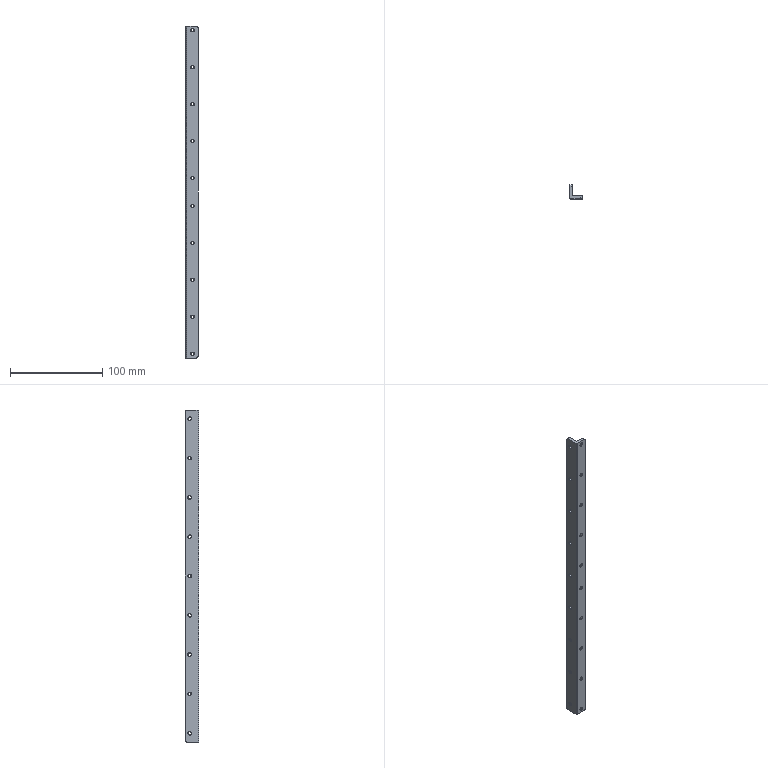Part | STEP file | L shaped aluminium angle 1 | 1 solid | 70 faces | box 13 x 15 x 359 mm | volume 26222 mm3 | cone 38 | cylinder 23 | plane 9 | commonest cylinder face diameters 3.3 x19 4 x4